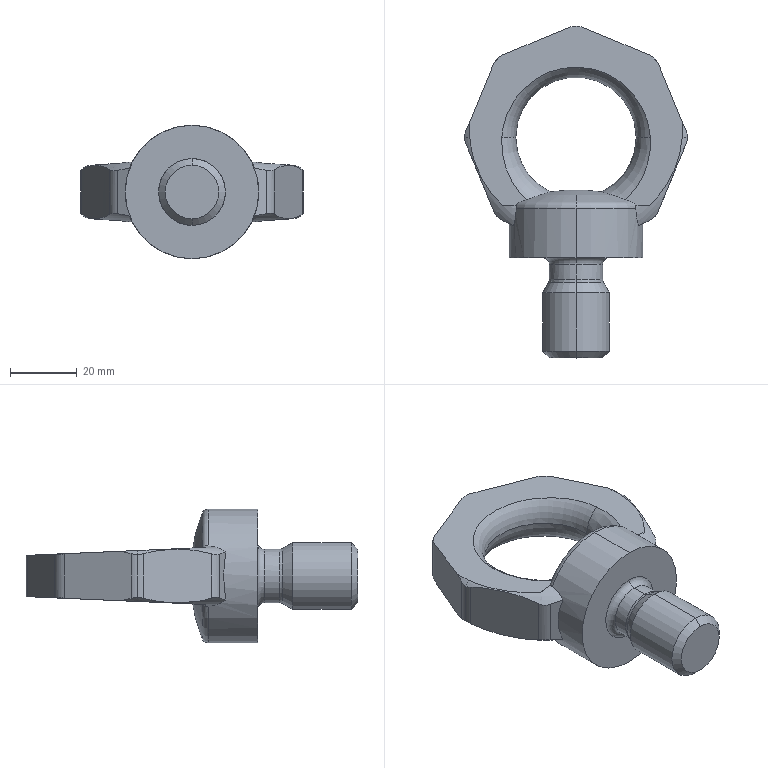Part | CATIA | 1 solid | 65 faces | box 66.676 x 99.338 x 40 mm | volume 54798 mm3 | torus 26 | plane 16 | cylinder 15 | sphere 4 | cone 4 | commonest cylinder face diameters 10 x9 16 x2 20 x2 40 x2